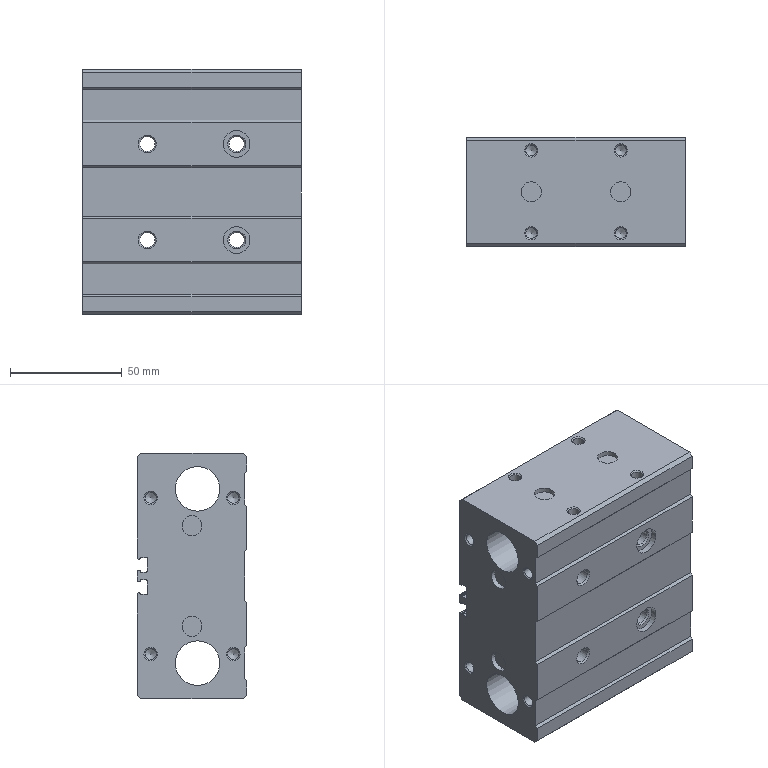Part | STEP file | 1 solid | 126 faces | box 98 x 49 x 110 mm | volume 384442 mm3 | plane 55 | cylinder 47 | cone 24 | commonest cylinder face diameters 0.4 x8 0.8 x8 4.917 x8 6.647 x4 8.566 x4 9 x4